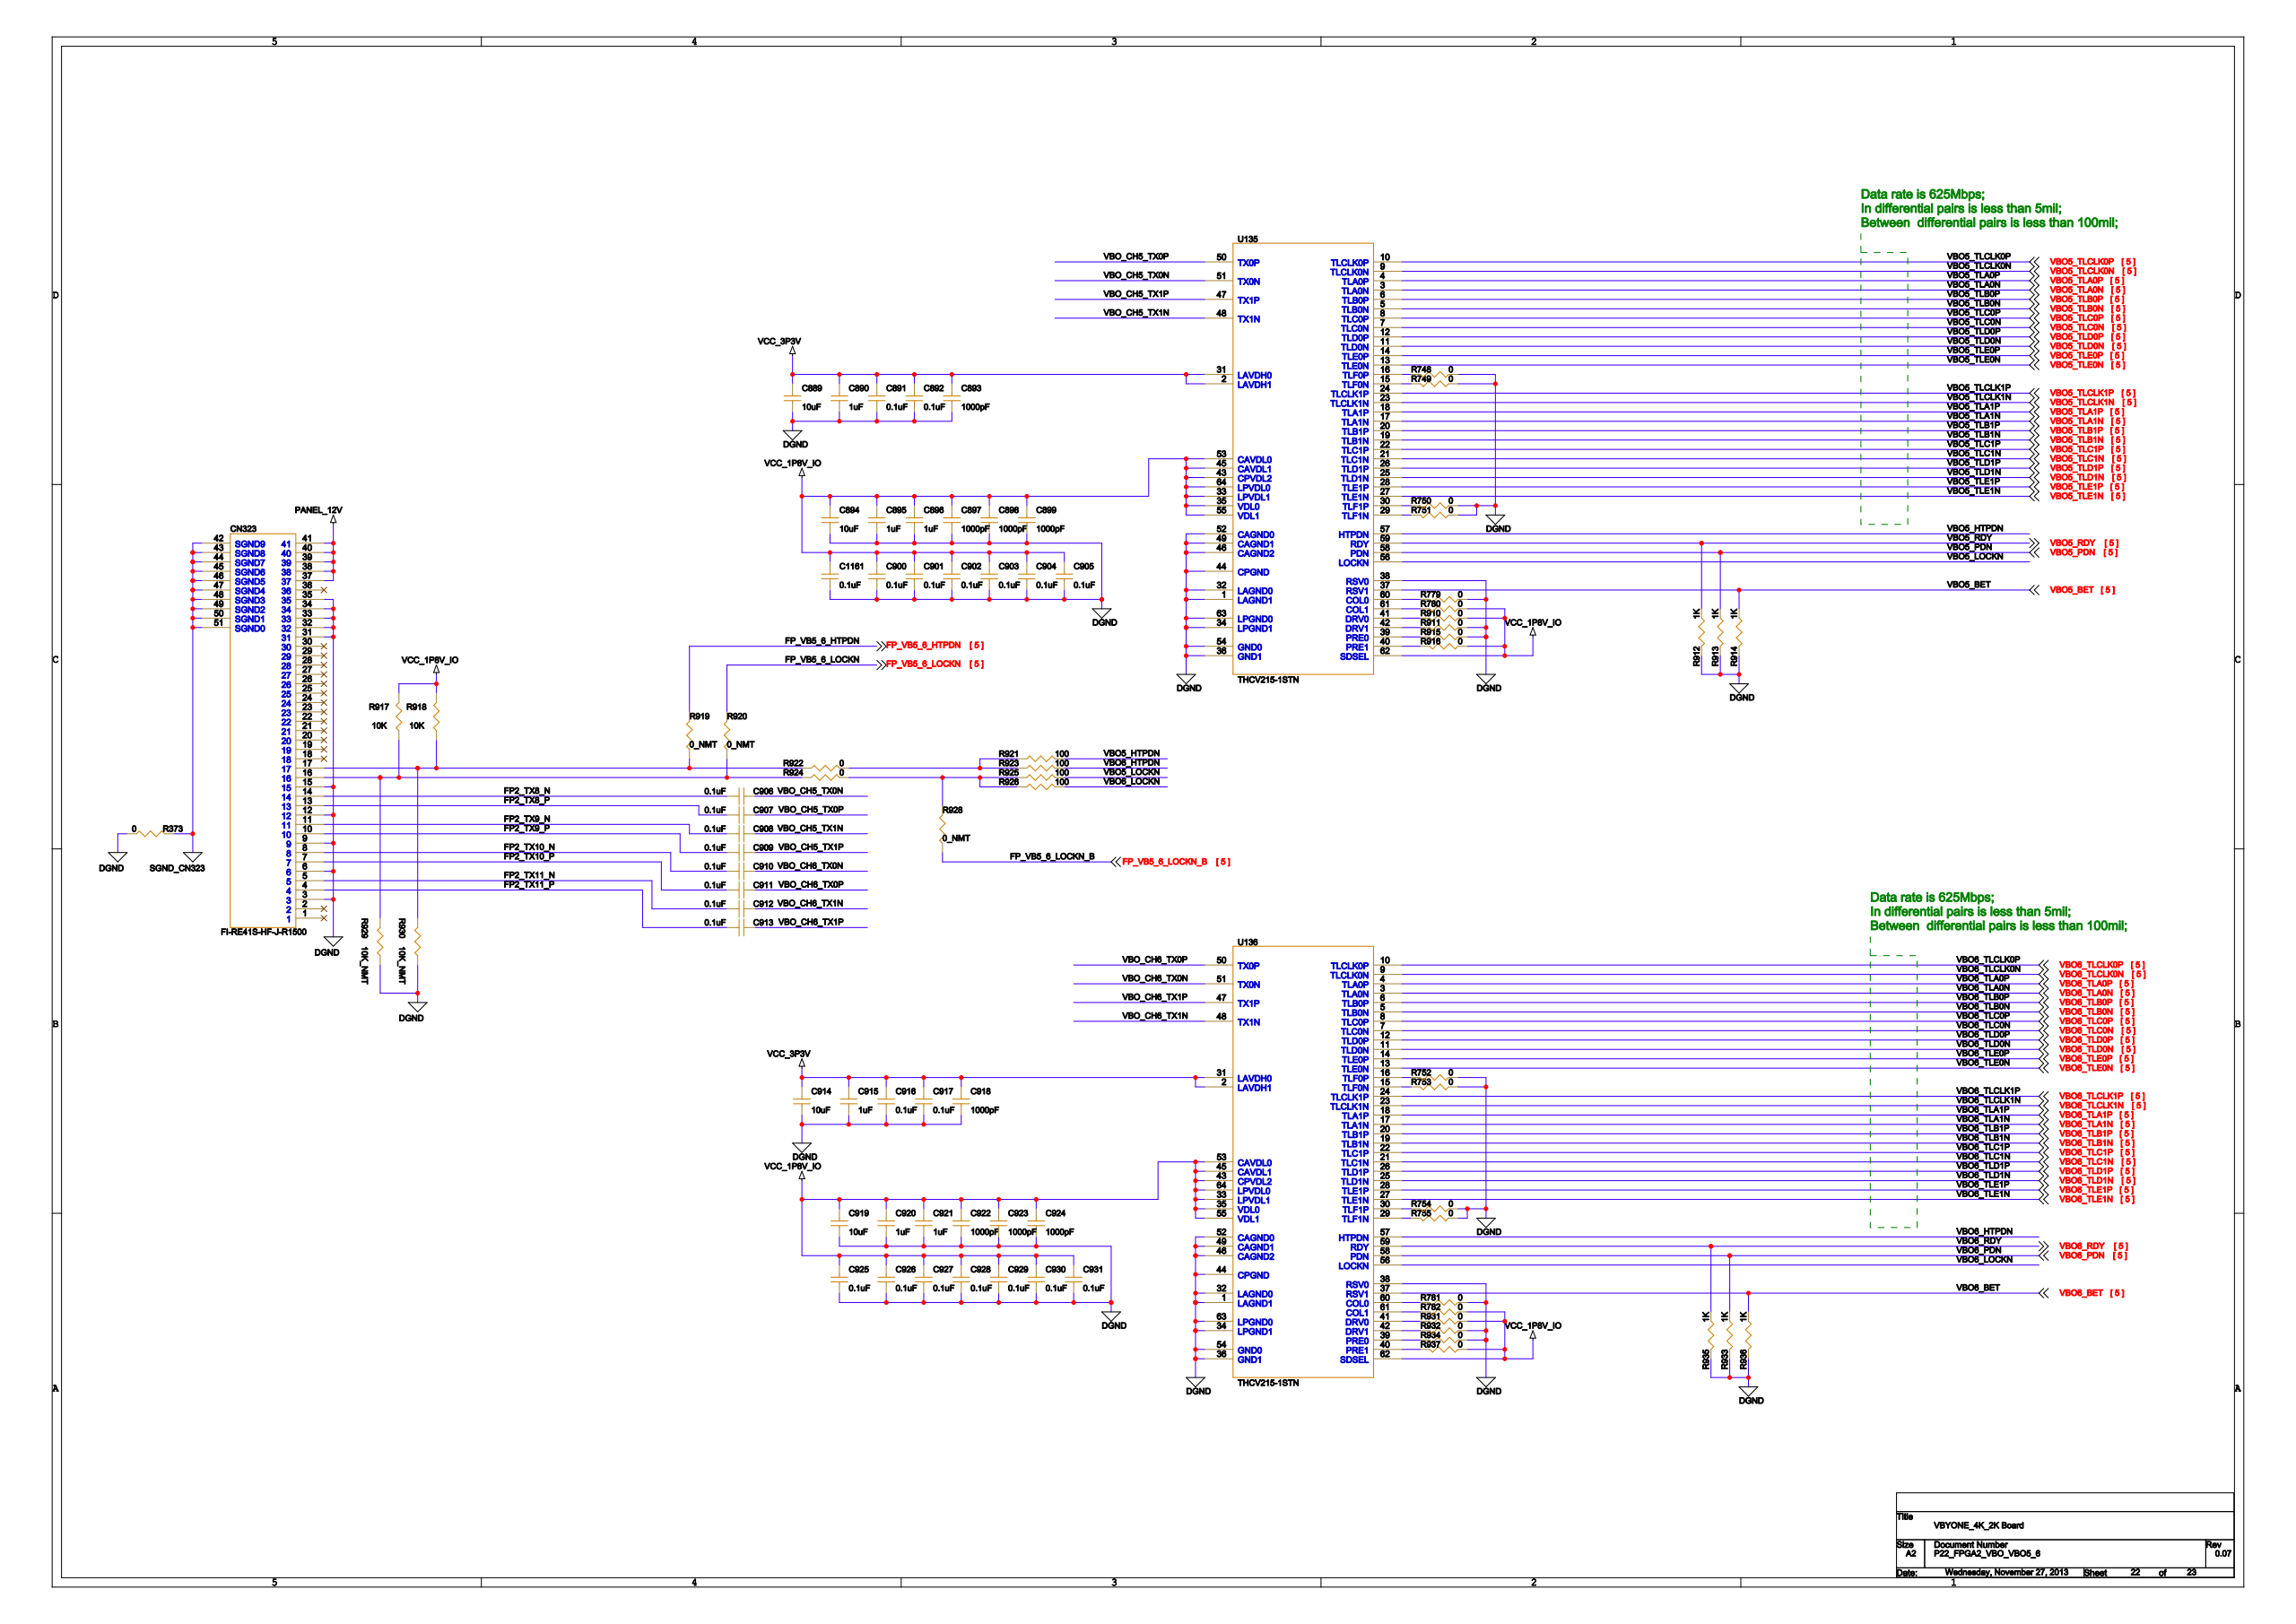Circuit board | Cadence Allegro | 1712 parts | 1495 nets | one sheet of the schematic
Parts on this sheet (reference | value | footprint):
C889 | 10uF | CRC2012RZAS
C890 | 1uF | CRC1608RZAS
C891 | 0.1uF | CRC1005RZAS
C892 | 0.1uF | CRC1005RZAS
C893 | 1000pF | CRC1608RZAS
C894 | 10uF | CRC2012RZAS
C895 | 1uF | CRC1608RZAS
C896 | 1uF | CRC1608RZAS
C897 | 1000pF | CRC1608RZAS
C898 | 1000pF | CRC1608RZAS
C899 | 1000pF | CRC1608RZAS
C900 | 0.1uF | CRC1005RZAS
C901 | 0.1uF | CRC1005RZAS
C902 | 0.1uF | CRC1005RZAS
C903 | 0.1uF | CRC1005RZAS
C904 | 0.1uF | CRC1005RZAS
C905 | 0.1uF | CRC1005RZAS
C906 | 0.1uF | CRC1005RZAS
C907 | 0.1uF | CRC1005RZAS
C908 | 0.1uF | CRC1005RZAS
C909 | 0.1uF | CRC1005RZAS
C910 | 0.1uF | CRC1005RZAS
C911 | 0.1uF | CRC1005RZAS
C912 | 0.1uF | CRC1005RZAS
C913 | 0.1uF | CRC1005RZAS
C914 | 10uF | CRC2012RZAS
C915 | 1uF | CRC1608RZAS
C916 | 0.1uF | CRC1005RZAS
C917 | 0.1uF | CRC1005RZAS
C918 | 1000pF | CRC1608RZAS
C919 | 10uF | CRC2012RZAS
C920 | 1uF | CRC1608RZAS
C921 | 1uF | CRC1608RZAS
C922 | 1000pF | CRC1608RZAS
C923 | 1000pF | CRC1608RZAS
C924 | 1000pF | CRC1608RZAS
C925 | 0.1uF | CRC1005RZAS
C926 | 0.1uF | CRC1005RZAS
C927 | 0.1uF | CRC1005RZAS
C928 | 0.1uF | CRC1005RZAS
C929 | 0.1uF | CRC1005RZAS
C930 | 0.1uF | CRC1005RZAS
C931 | 0.1uF | CRC1005RZAS
C1161 | 0.1uF | CRC1005RZAS
CN323 | FI-RE41S-HF-J-R1500 | CAC041RCAS
R373 | 0 | CRC1608RZAS
R748 | 0 | CRC1608RZAS
R749 | 0 | CRC1608RZAS
R750 | 0 | CRC1608RZAS
R751 | 0 | CRC1608RZAS
R752 | 0 | CRC1608RZAS
R753 | 0 | CRC1608RZAS
R754 | 0 | CRC1608RZAS
R755 | 0 | CRC1608RZAS
R779 | 0 | CRC1608RZAS
R780 | 0 | CRC1608RZAS
R781 | 0 | CRC1608RZAS
R782 | 0 | CRC1608RZAS
R910 | 0 | CRC1608RZAS
R911 | 0 | CRC1608RZAS
R912 | 1K | CRC1608RZAS
R913 | 1K | CRC1608RZAS
R914 | 1K | CRC1608RZAS
R915 | 0 | CRC1608RZAS
R916 | 0 | CRC1608RZAS
R917 | 10K | CRC1005RZAS
R918 | 10K | CRC1005RZAS
R919 | 0_NMT | CRC1608RZAS
R920 | 0_NMT | CRC1608RZAS
R921 | 100 | CRC1005RZAS
R922 | 0 | CRC1608RZAS
R923 | 100 | CRC1005RZAS
R924 | 0 | CRC1608RZAS
R925 | 100 | CRC1005RZAS
R926 | 100 | CRC1005RZAS
R928 | 0_NMT | CRC1608RZAS
R929 | 10K_NMT | CRC1005RZAS
R930 | 10K_NMT | CRC1005RZAS
R931 | 0 | CRC1608RZAS
R932 | 0 | CRC1608RZAS
R933 | 1K | CRC1608RZAS
R934 | 0 | CRC1608RZAS
R935 | 1K | CRC1608RZAS
R936 | 1K | CRC1608RZAS
R937 | 0 | CRC1608RZAS
U135 | THCV215-1STN | SOC064RCAT
U136 | THCV215-1STN | SOC064RCAT
Nets of these parts (net: part-pin ...):
VCC_3P3V: C889-2 C890-2 C891-2 C892-2 C893-2 C914-2 C915-2 C916-2 C917-2 C918-2 U135-2 U135-31 U136-2 U136-31
DGND: C889-1 C890-1 C891-1 C892-1 C893-1 C894-1 C895-1 C896-1 C897-1 C898-1 C899-1 C900-1 C901-1 C902-1 C903-1 C904-1 C905-1 C914-1 C915-1 C916-1 C917-1 C918-1 C919-1 C920-1 C921-1 C922-1 C923-1 C924-1 C925-1 C926-1 C927-1 C928-1 C929-1 C930-1 C931-1 C1161-1 R373-2 R748-2 R749-2 R750-2 R751-2 R752-2 R753-2 R754-2 R755-2 R779-2 R781-2 R911-2 R912-1 R913-1 R914-1 R915-2 R929-2 R930-2 R932-2 R933-1 R934-2 R935-1 R936-1 CN323-3 CN323-6 CN323-9 CN323-12 CN323-15 CN323-31 CN323-32 CN323-33 CN323-34 CN323-35 U135-1 U135-32 U135-34 U135-36 U135-38 U135-44 U135-46 U135-49 U135-52 U135-54 U135-63 U136-1 U136-32 U136-34 U136-36 U136-38 U136-44 U136-46 U136-49 U136-52 U136-54 U136-63
VCC_1P8V_IO: C894-2 C895-2 C896-2 C897-2 C898-2 C899-2 C900-2 C901-2 C902-2 C903-2 C904-2 C905-2 C919-2 C920-2 C921-2 C922-2 C923-2 C924-2 C925-2 C926-2 C927-2 C928-2 C929-2 C930-2 C931-2 C1161-2 R780-2 R782-2 R910-2 R916-2 R917-1 R918-1 R931-2 R937-2 U135-33 U135-35 U135-43 U135-45 U135-53 U135-55 U135-62 U135-64 U136-33 U136-35 U136-43 U136-45 U136-53 U136-55 U136-62 U136-64
PANEL_12V: CN323-37 CN323-38 CN323-39 CN323-40 CN323-41
VBO_CH5_TX0N: C906-1 U135-51
FP2_TX8_N: C906-2 CN323-14
VBO_CH5_TX0P: C907-1 U135-50
FP2_TX8_P: C907-2 CN323-13
VBO_CH5_TX1N: C908-1 U135-48
FP2_TX9_N: C908-2 CN323-11
VBO_CH5_TX1P: C909-1 U135-47
FP2_TX9_P: C909-2 CN323-10
VBO_CH6_TX0N: C910-1 U136-51
FP2_TX10_N: C910-2 CN323-8
VBO_CH6_TX0P: C911-1 U136-50
FP2_TX10_P: C911-2 CN323-7
VBO_CH6_TX1N: C912-1 U136-48
FP2_TX11_N: C912-2 CN323-5
VBO_CH6_TX1P: C913-1 U136-47
FP2_TX11_P: C913-2 CN323-4
SGND_CN323: R373-1 CN323-42 CN323-43 CN323-44 CN323-45 CN323-46 CN323-47 CN323-48 CN323-49 CN323-50 CN323-51
N19770819: R917-2 R920-2 R924-2 R929-1 CN323-16
N19770817: R918-2 R919-2 R922-2 R930-1 CN323-17
N19770908: R921-2 R922-1 R923-2
N19770910: R924-1 R925-2 R926-2 R928-1
FP_VB5_6_HTPDN: R919-1
FP_VB5_6_LOCKN: R920-1
FP_VB5_6_LOCKN_B: R928-2
VBO5_HTPDN: R921-1 U135-57
VBO6_HTPDN: R923-1 U136-57
VBO5_LOCKN: R925-1 U135-56
VBO6_LOCKN: R926-1 U136-56
VBO5_RDY: R912-2 U135-59
VBO5_PDN: R913-2 U135-58
VBO5_BET: R914-2 U135-37
VBO6_PDN: R933-2 U136-58
VBO6_RDY: R935-2 U136-59
VBO6_BET: R936-2 U136-37
N19923785: R748-1 U135-16
N19923775: R749-1 U135-15
N19928220: R750-1 U135-30
N19928221: R751-1 U135-29
N19924086: R752-1 U136-16
N19924076: R753-1 U136-15
N19927437: R754-1 U136-30
N19927438: R755-1 U136-29
N20036306: R779-1 U135-60
N20036501: R780-1 U135-61
N20036941: R781-1 U136-60
N20037136: R782-1 U136-61
N19771684: R910-1 U135-41
N19771682: R911-1 U135-42
N19771690: R915-1 U135-39
N19771694: R916-1 U135-40
N20038533: R931-1 U136-41
N20038537: R932-1 U136-42
N20038548: R934-1 U136-39
N20038551: R937-1 U136-40
VBO6_TLB0P: U136-6
VBO6_TLB0N: U136-5
VBO6_TLA0P: U136-4
VBO5_TLA0P: U135-4
VBO5_TLC0P: U135-8
VBO5_TLC0N: U135-7
VBO6_TLC0P: U136-8
VBO6_TLC0N: U136-7
VBO6_TLC1P: U136-22
VBO6_TLD1P: U136-26
VBO6_TLD1N: U136-25
VBO6_TLA0N: U136-3
VBO5_TLA0N: U135-3
VBO5_TLD0P: U135-12
VBO5_TLD0N: U135-11
VBO6_TLD0P: U136-12
VBO6_TLD0N: U136-11
VBO6_TLC1N: U136-21
VBO6_TLB1P: U136-20
VBO6_TLB1N: U136-19
VBO5_TLB1P: U135-20
VBO5_TLCLK1P: U135-24
VBO5_TLCLK1N: U135-23
VBO6_TLCLK0P: U136-10
VBO6_TLCLK0N: U136-9
VBO6_TLA1P: U136-18
VBO6_TLA1N: U136-17
VBO5_TLB1N: U135-19
VBO5_TLD1P: U135-26
VBO5_TLD1N: U135-25
VBO5_TLE1P: U135-28
VBO5_TLE1N: U135-27
VBO6_TLE0P: U136-14
VBO6_TLE0N: U136-13
VBO6_TLCLK1P: U136-24
VBO5_TLCLK0P: U135-10
VBO5_TLE0P: U135-14
VBO5_TLE0N: U135-13
VBO5_TLC1P: U135-22
VBO5_TLC1N: U135-21
VBO6_TLCLK1N: U136-23
VBO5_TLCLK0N: U135-9
VBO5_TLB0P: U135-6
VBO5_TLB0N: U135-5
VBO5_TLA1P: U135-18
VBO5_TLA1N: U135-17
VBO6_TLE1P: U136-28
VBO6_TLE1N: U136-27